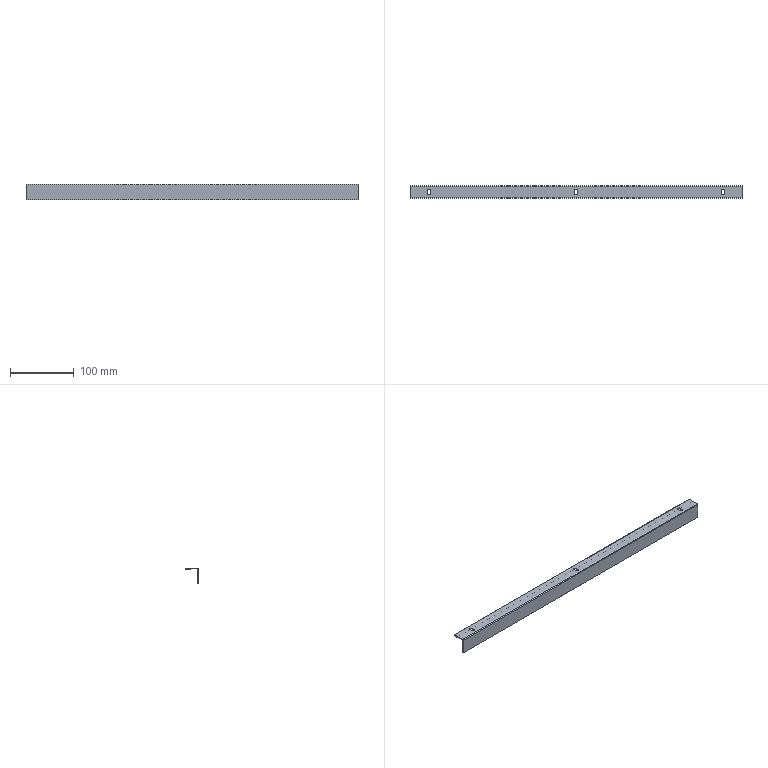Part | STEP file | HESS-408-70-15W-N-20-inner liner louver lower baffle | 1 solid | 34 faces | box 519 x 20 x 25 mm | volume 26517 mm3 | plane 19 | cylinder 15 | commonest cylinder face diameters 5 x6 6.5 x3 0.1 x2 2.1 x2 0.2 x1 2.2 x1